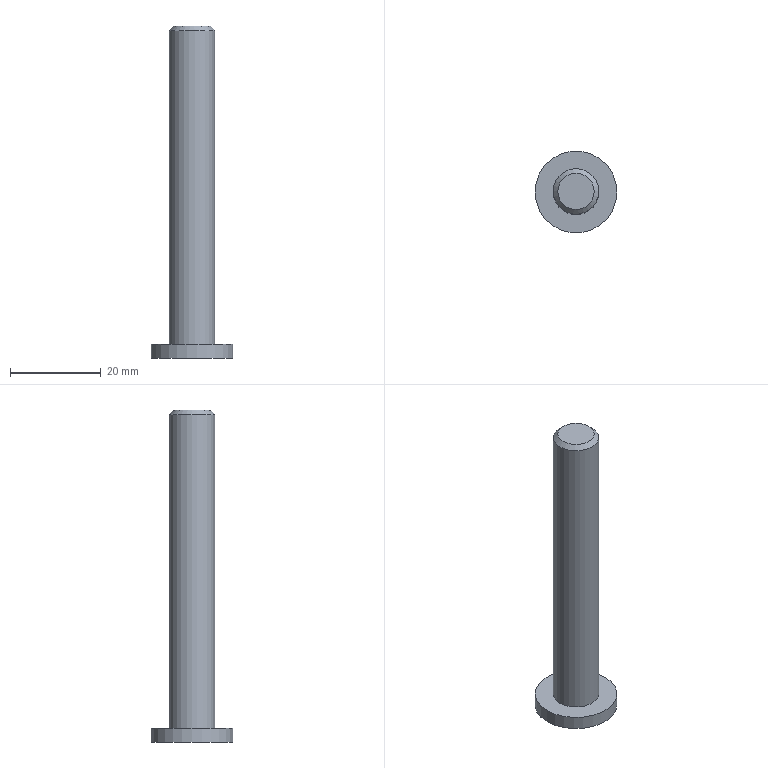Part | NX | features BREP 1, DATUM_CSYS 1 | 1 solid | 9 faces | box 18 x 18 x 73 mm | volume 5726 mm3 | cylinder 4 | plane 3 | cone 2 | commonest cylinder face diameters 5 x2 10 x1 18 x1
STEP:
#1=CARTESIAN_POINT('',(9.,0.,-3.));
#2=VERTEX_POINT('',#1);
#3=CARTESIAN_POINT('',(0.,0.,-3.));
#4=DIRECTION('',(0.,0.,-1.));
#5=DIRECTION('',(1.,0.,0.));
#6=AXIS2_PLACEMENT_3D('',#3,#4,#5);
#7=CIRCLE('',#6,9.);
#8=EDGE_CURVE('',#2,#2,#7,.T.);
#9=ORIENTED_EDGE('',*,*,#8,.T.);
#10=EDGE_LOOP('',(#9));
#11=FACE_BOUND('',#10,.T.);
#12=CARTESIAN_POINT('',(2.5,0.,-3.));
#13=VERTEX_POINT('',#12);
#14=CARTESIAN_POINT('',(0.,0.,-3.));
#15=DIRECTION('',(0.,0.,1.));
#16=DIRECTION('',(1.,0.,0.));
#17=AXIS2_PLACEMENT_3D('',#14,#15,#16);
#18=CIRCLE('',#17,2.5);
#19=EDGE_CURVE('',#13,#13,#18,.T.);
#20=ORIENTED_EDGE('',*,*,#19,.T.);
#21=EDGE_LOOP('',(#20));
#22=FACE_BOUND('',#21,.T.);
#23=CARTESIAN_POINT('',(0.,0.,-3.));
#24=DIRECTION('',(0.,0.,-1.));
#25=DIRECTION('',(-1.,0.,0.));
#26=AXIS2_PLACEMENT_3D('',#23,#24,#25);
#27=PLANE('',#26);
#28=ADVANCED_FACE('',(#11,#22),#27,.T.);
#29=CARTESIAN_POINT('',(9.,0.,0.));
#30=VERTEX_POINT('',#29);
#31=CARTESIAN_POINT('',(0.,0.,0.));
#32=DIRECTION('',(0.,0.,-1.));
#33=DIRECTION('',(1.,0.,0.));
#34=AXIS2_PLACEMENT_3D('',#31,#32,#33);
#35=CIRCLE('',#34,9.);
#36=EDGE_CURVE('',#30,#30,#35,.T.);
#37=ORIENTED_EDGE('',*,*,#36,.T.);
#38=CARTESIAN_POINT('',(9.,0.,0.));
#39=DIRECTION('',(0.,0.,-1.));
#40=VECTOR('',#39,1000.);
#41=LINE('',#38,#40);
#42=EDGE_CURVE('',#30,#2,#41,.T.);
#43=ORIENTED_EDGE('',*,*,#42,.T.);
#44=ORIENTED_EDGE('',*,*,#8,.F.);
#45=ORIENTED_EDGE('',*,*,#42,.F.);
#46=EDGE_LOOP('',(#37,#43,#44,#45));
#47=FACE_BOUND('',#46,.T.);
#48=CARTESIAN_POINT('',(0.,0.,0.));
#49=DIRECTION('',(0.,0.,-1.));
#50=DIRECTION('',(-1.,0.,0.));
#51=AXIS2_PLACEMENT_3D('',#48,#49,#50);
#52=CYLINDRICAL_SURFACE('',#51,9.);
#53=ADVANCED_FACE('',(#47),#52,.T.);
#54=ORIENTED_EDGE('',*,*,#36,.F.);
#55=EDGE_LOOP('',(#54));
#56=FACE_BOUND('',#55,.T.);
#57=CARTESIAN_POINT('',(5.,0.,0.));
#58=VERTEX_POINT('',#57);
#59=CARTESIAN_POINT('',(0.,0.,0.));
#60=DIRECTION('',(0.,0.,1.));
#61=DIRECTION('',(1.,0.,0.));
#62=AXIS2_PLACEMENT_3D('',#59,#60,#61);
#63=CIRCLE('',#62,5.);
#64=EDGE_CURVE('',#58,#58,#63,.T.);
#65=ORIENTED_EDGE('',*,*,#64,.F.);
#66=EDGE_LOOP('',(#65));
#67=FACE_BOUND('',#66,.T.);
#68=CARTESIAN_POINT('',(0.,0.,0.));
#69=DIRECTION('',(0.,0.,-1.));
#70=DIRECTION('',(-1.,0.,0.));
#71=AXIS2_PLACEMENT_3D('',#68,#69,#70);
#72=PLANE('',#71);
#73=ADVANCED_FACE('',(#56,#67),#72,.F.);
#74=ORIENTED_EDGE('',*,*,#64,.T.);
#75=CARTESIAN_POINT('',(5.,0.,69.));
#76=VERTEX_POINT('',#75);
#77=CARTESIAN_POINT('',(5.,0.,0.));
#78=DIRECTION('',(0.,0.,1.));
#79=VECTOR('',#78,1000.);
#80=LINE('',#77,#79);
#81=EDGE_CURVE('',#58,#76,#80,.T.);
#82=ORIENTED_EDGE('',*,*,#81,.T.);
#83=CARTESIAN_POINT('',(0.,0.,69.));
#84=DIRECTION('',(0.,0.,-1.));
#85=DIRECTION('',(1.,0.,0.));
#86=AXIS2_PLACEMENT_3D('',#83,#84,#85);
#87=CIRCLE('',#86,5.);
#88=EDGE_CURVE('',#76,#76,#87,.T.);
#89=ORIENTED_EDGE('',*,*,#88,.T.);
#90=ORIENTED_EDGE('',*,*,#81,.F.);
#91=EDGE_LOOP('',(#74,#82,#89,#90));
#92=FACE_BOUND('',#91,.T.);
#93=CARTESIAN_POINT('',(0.,0.,0.));
#94=DIRECTION('',(0.,0.,1.));
#95=DIRECTION('',(-1.,0.,0.));
#96=AXIS2_PLACEMENT_3D('',#93,#94,#95);
#97=CYLINDRICAL_SURFACE('',#96,5.);
#98=ADVANCED_FACE('',(#92),#97,.T.);
#99=CARTESIAN_POINT('',(4.,0.,70.));
#100=VERTEX_POINT('',#99);
#101=CARTESIAN_POINT('',(0.,0.,70.));
#102=DIRECTION('',(0.,0.,-1.));
#103=DIRECTION('',(1.,0.,0.));
#104=AXIS2_PLACEMENT_3D('',#101,#102,#103);
#105=CIRCLE('',#104,4.);
#106=EDGE_CURVE('',#100,#100,#105,.T.);
#107=ORIENTED_EDGE('',*,*,#106,.F.);
#108=EDGE_LOOP('',(#107));
#109=FACE_BOUND('',#108,.T.);
#110=CARTESIAN_POINT('',(0.,0.,70.));
#111=DIRECTION('',(0.,0.,1.));
#112=DIRECTION('',(-1.,0.,0.));
#113=AXIS2_PLACEMENT_3D('',#110,#111,#112);
#114=PLANE('',#113);
#115=ADVANCED_FACE('',(#109),#114,.T.);
#116=CARTESIAN_POINT('',(4.,0.,70.));
#117=DIRECTION('',(0.7071,0.,-0.7071));
#118=VECTOR('',#117,1000.);
#119=LINE('',#116,#118);
#120=EDGE_CURVE('',#100,#76,#119,.T.);
#121=ORIENTED_EDGE('',*,*,#120,.T.);
#122=ORIENTED_EDGE('',*,*,#88,.F.);
#123=ORIENTED_EDGE('',*,*,#120,.F.);
#124=ORIENTED_EDGE('',*,*,#106,.T.);
#125=EDGE_LOOP('',(#121,#122,#123,#124));
#126=FACE_BOUND('',#125,.T.);
#127=CARTESIAN_POINT('',(0.,0.,70.));
#128=DIRECTION('',(0.,0.,-1.));
#129=DIRECTION('',(-1.,0.,0.));
#130=AXIS2_PLACEMENT_3D('',#127,#128,#129);
#131=CONICAL_SURFACE('',#130,4.,0.7854);
#132=ADVANCED_FACE('',(#126),#131,.T.);
#133=CARTESIAN_POINT('',(2.5,0.,21.));
#134=VERTEX_POINT('',#133);
#135=CARTESIAN_POINT('',(2.5,0.,-3.));
#136=DIRECTION('',(0.,0.,1.));
#137=VECTOR('',#136,1000.);
#138=LINE('',#135,#137);
#139=EDGE_CURVE('',#13,#134,#138,.T.);
#140=ORIENTED_EDGE('',*,*,#139,.T.);
#141=CARTESIAN_POINT('',(0.,0.,21.));
#142=DIRECTION('',(0.,0.,1.));
#143=DIRECTION('',(1.,0.,0.));
#144=AXIS2_PLACEMENT_3D('',#141,#142,#143);
#145=CIRCLE('',#144,2.5);
#146=EDGE_CURVE('',#134,#134,#145,.T.);
#147=ORIENTED_EDGE('',*,*,#146,.T.);
#148=ORIENTED_EDGE('',*,*,#139,.F.);
#149=ORIENTED_EDGE('',*,*,#19,.F.);
#150=EDGE_LOOP('',(#140,#147,#148,#149));
#151=FACE_BOUND('',#150,.T.);
#152=CARTESIAN_POINT('',(0.,0.,-3.));
#153=DIRECTION('',(0.,0.,1.));
#154=DIRECTION('',(-1.,0.,0.));
#155=AXIS2_PLACEMENT_3D('',#152,#153,#154);
#156=CYLINDRICAL_SURFACE('',#155,2.5);
#157=ADVANCED_FACE('',(#151),#156,.F.);
#158=CARTESIAN_POINT('',(2.5,0.,23.));
#159=VERTEX_POINT('',#158);
#160=CARTESIAN_POINT('',(2.5,0.,21.));
#161=DIRECTION('',(0.,0.,1.));
#162=VECTOR('',#161,1000.);
#163=LINE('',#160,#162);
#164=EDGE_CURVE('',#134,#159,#163,.T.);
#165=ORIENTED_EDGE('',*,*,#164,.T.);
#166=CARTESIAN_POINT('',(0.,0.,23.));
#167=DIRECTION('',(0.,0.,1.));
#168=DIRECTION('',(1.,0.,0.));
#169=AXIS2_PLACEMENT_3D('',#166,#167,#168);
#170=CIRCLE('',#169,2.5);
#171=EDGE_CURVE('',#159,#159,#170,.T.);
#172=ORIENTED_EDGE('',*,*,#171,.T.);
#173=ORIENTED_EDGE('',*,*,#164,.F.);
#174=ORIENTED_EDGE('',*,*,#146,.F.);
#175=EDGE_LOOP('',(#165,#172,#173,#174));
#176=FACE_BOUND('',#175,.T.);
#177=CARTESIAN_POINT('',(0.,0.,21.));
#178=DIRECTION('',(0.,0.,1.));
#179=DIRECTION('',(-1.,0.,0.));
#180=AXIS2_PLACEMENT_3D('',#177,#178,#179);
#181=CYLINDRICAL_SURFACE('',#180,2.5);
#182=ADVANCED_FACE('',(#176),#181,.F.);
#183=CARTESIAN_POINT('',(0.,0.,24.502));
#184=VERTEX_POINT('',#183);
#185=CARTESIAN_POINT('',(2.5,0.,23.));
#186=DIRECTION('',(-0.8572,0.,0.515));
#187=VECTOR('',#186,1000.);
#188=LINE('',#185,#187);
#189=EDGE_CURVE('',#159,#184,#188,.T.);
#190=ORIENTED_EDGE('',*,*,#189,.T.);
#191=ORIENTED_EDGE('',*,*,#189,.F.);
#192=ORIENTED_EDGE('',*,*,#171,.F.);
#193=EDGE_LOOP('',(#190,#191,#192));
#194=FACE_BOUND('',#193,.T.);
#195=CARTESIAN_POINT('',(0.,0.,24.502));
#196=DIRECTION('',(0.,0.,-1.));
#197=DIRECTION('',(-1.,0.,0.));
#198=AXIS2_PLACEMENT_3D('',#195,#196,#197);
#199=CONICAL_SURFACE('',#198,0.,1.03);
#200=ADVANCED_FACE('',(#194),#199,.F.);
#201=CLOSED_SHELL('',(#28,#53,#73,#98,#115,#132,#157,#182,#200));
#202=MANIFOLD_SOLID_BREP('',#201);
#203=(LENGTH_UNIT()NAMED_UNIT(*)SI_UNIT(.MILLI.,.METRE.));
#204=UNCERTAINTY_MEASURE_WITH_UNIT(LENGTH_MEASURE(0.00001),#203,'','');
#205=(NAMED_UNIT(*)PLANE_ANGLE_UNIT()SI_UNIT($,.RADIAN.));
#206=(NAMED_UNIT(*)SI_UNIT($,.STERADIAN.)SOLID_ANGLE_UNIT());
#207=(GEOMETRIC_REPRESENTATION_CONTEXT(3)GLOBAL_UNCERTAINTY_ASSIGNED_CONTEXT((#204))GLOBAL_UNIT_ASSIGNED_CONTEXT((#203,#205,#206))REPRESENTATION_CONTEXT('',''));
#208=ADVANCED_BREP_SHAPE_REPRESENTATION('',(#202),#207);